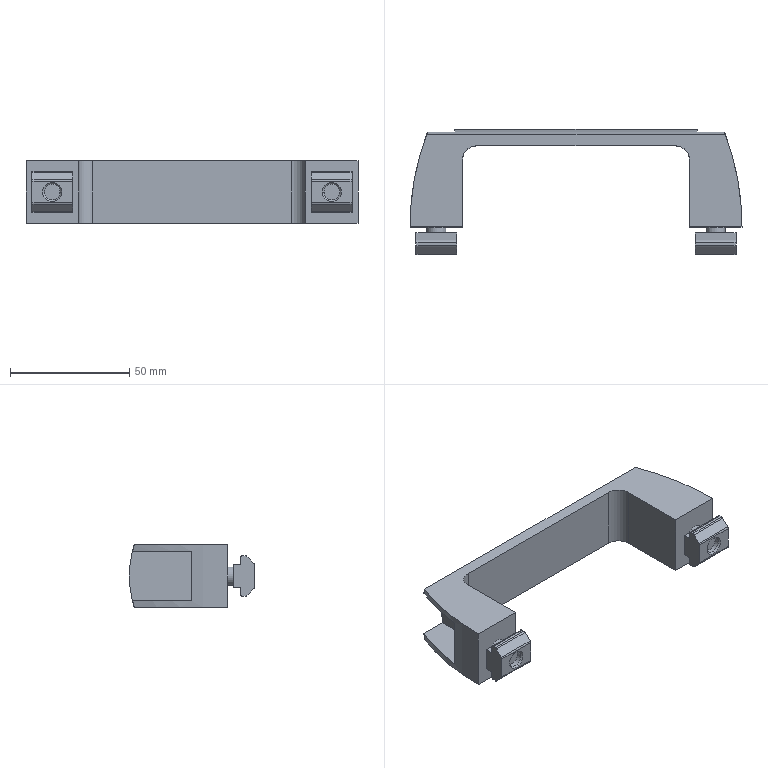Part | STEP file | UPCN26-M-41-SET | 5 solids | 114 faces | box 139 x 52.5 x 26 mm | volume 44539 mm3 | plane 71 | cylinder 31 | cone 10 | torus 2 | commonest cylinder face diameters 2 x12 6 x4 6.647 x2 8 x2 8.5 x2 12 x2